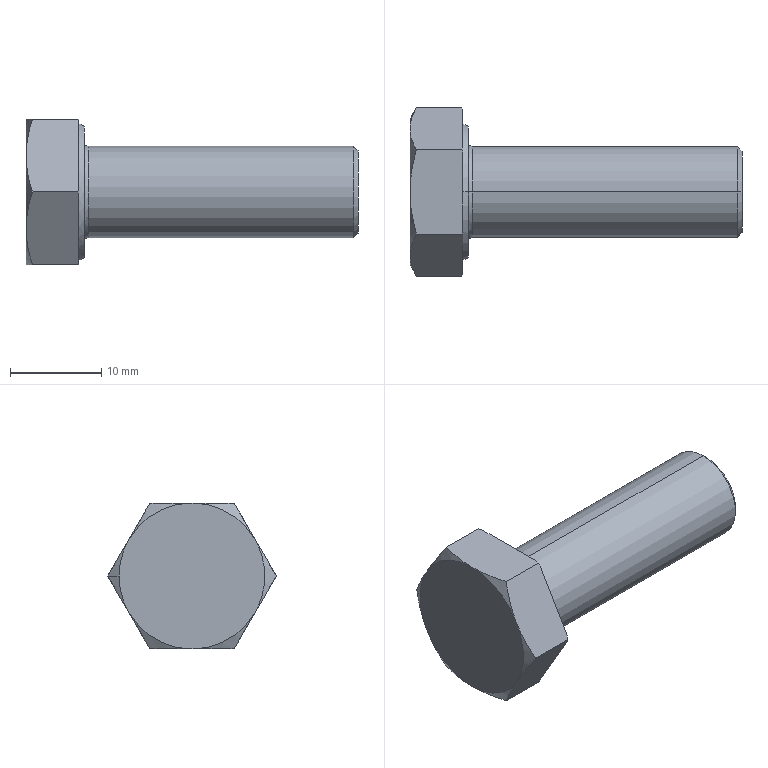Part | SolidWorks | features BaseBody 1, Chamfer 1, ICE 1 | 1 solid | 31 faces | box 36.4 x 18.475 x 16 mm | volume 3737 mm3 | cone 17 | plane 10 | spline 2 | cylinder 2 | commonest cylinder face diameters 10 x2
STEP:
#1=CARTESIAN_POINT('',(6.8,0.,-5.));
#2=VERTEX_POINT('',#1);
#3=CARTESIAN_POINT('',(6.8,0.,5.));
#4=VERTEX_POINT('',#3);
#5=CARTESIAN_POINT('',(6.8,0.,0.));
#6=DIRECTION('',(1.,0.,0.));
#7=DIRECTION('',(0.,0.,-1.));
#8=AXIS2_PLACEMENT_3D('',#5,#6,#7);
#9=CIRCLE('',#8,5.);
#10=EDGE_CURVE('',#2,#4,#9,.T.);
#11=ORIENTED_EDGE('',*,*,#10,.F.);
#12=CARTESIAN_POINT('',(6.4,0.,-5.4));
#13=VERTEX_POINT('',#12);
#14=CARTESIAN_POINT('',(6.8,0.,-5.4));
#15=DIRECTION('',(0.,-1.,0.));
#16=DIRECTION('',(0.,0.,-1.));
#17=AXIS2_PLACEMENT_3D('',#14,#15,#16);
#18=CIRCLE('',#17,0.4);
#19=EDGE_CURVE('',#2,#13,#18,.T.);
#20=ORIENTED_EDGE('',*,*,#19,.T.);
#21=CARTESIAN_POINT('',(6.4,0.,5.4));
#22=VERTEX_POINT('',#21);
#23=CARTESIAN_POINT('',(6.4,0.,5.4));
#24=CARTESIAN_POINT('',(6.4,0.1651,5.4));
#25=CARTESIAN_POINT('',(6.4,0.4117,5.389));
#26=CARTESIAN_POINT('',(6.4,0.6977,5.356));
#27=CARTESIAN_POINT('',(6.4,0.8403,5.334));
#28=CARTESIAN_POINT('',(6.4,0.9013,5.324));
#29=CARTESIAN_POINT('',(6.4,0.942,5.317));
#30=CARTESIAN_POINT('',(6.4,0.9611,5.314));
#31=CARTESIAN_POINT('',(6.4,1.155,5.278));
#32=CARTESIAN_POINT('',(6.4,1.409,5.218));
#33=CARTESIAN_POINT('',(6.4,1.7,5.127));
#34=CARTESIAN_POINT('',(6.4,1.824,5.083));
#35=CARTESIAN_POINT('',(6.4,1.906,5.053));
#36=CARTESIAN_POINT('',(6.4,1.945,5.038));
#37=CARTESIAN_POINT('',(6.4,2.157,4.954));
#38=CARTESIAN_POINT('',(6.4,2.405,4.841));
#39=CARTESIAN_POINT('',(6.4,2.644,4.709));
#40=CARTESIAN_POINT('',(6.4,2.801,4.618));
#41=CARTESIAN_POINT('',(6.4,2.877,4.571));
#42=CARTESIAN_POINT('',(6.4,3.267,4.316));
#43=CARTESIAN_POINT('',(6.4,3.555,4.082));
#44=CARTESIAN_POINT('',(6.4,3.95,3.687));
#45=CARTESIAN_POINT('',(6.4,4.137,3.48));
#46=CARTESIAN_POINT('',(6.4,4.306,3.26));
#47=CARTESIAN_POINT('',(6.4,4.416,3.11));
#48=CARTESIAN_POINT('',(6.4,4.47,3.031));
#49=CARTESIAN_POINT('',(6.4,4.62,2.802));
#50=CARTESIAN_POINT('',(6.4,4.757,2.567));
#51=CARTESIAN_POINT('',(6.4,4.896,2.281));
#52=CARTESIAN_POINT('',(6.4,4.951,2.156));
#53=CARTESIAN_POINT('',(6.4,4.987,2.072));
#54=CARTESIAN_POINT('',(6.4,5.005,2.028));
#55=CARTESIAN_POINT('',(6.4,5.085,1.825));
#56=CARTESIAN_POINT('',(6.4,5.17,1.577));
#57=CARTESIAN_POINT('',(6.4,5.247,1.282));
#58=CARTESIAN_POINT('',(6.4,5.28,1.133));
#59=CARTESIAN_POINT('',(6.4,5.293,1.069));
#60=CARTESIAN_POINT('',(6.4,5.302,1.026));
#61=CARTESIAN_POINT('',(6.4,5.306,1.003));
#62=CARTESIAN_POINT('',(6.4,5.37,0.6582));
#63=CARTESIAN_POINT('',(6.4,5.4,0.3299));
#64=CARTESIAN_POINT('',(6.4,5.4,-0.165));
#65=CARTESIAN_POINT('',(6.4,5.389,-0.4115));
#66=CARTESIAN_POINT('',(6.4,5.356,-0.6976));
#67=CARTESIAN_POINT('',(6.4,5.335,-0.8402));
#68=CARTESIAN_POINT('',(6.4,5.324,-0.9013));
#69=CARTESIAN_POINT('',(6.4,5.317,-0.9419));
#70=CARTESIAN_POINT('',(6.4,5.314,-0.9611));
#71=CARTESIAN_POINT('',(6.4,5.278,-1.155));
#72=CARTESIAN_POINT('',(6.4,5.218,-1.409));
#73=CARTESIAN_POINT('',(6.4,5.127,-1.7));
#74=CARTESIAN_POINT('',(6.4,5.083,-1.824));
#75=CARTESIAN_POINT('',(6.4,5.053,-1.906));
#76=CARTESIAN_POINT('',(6.4,5.038,-1.945));
#77=CARTESIAN_POINT('',(6.4,4.954,-2.157));
#78=CARTESIAN_POINT('',(6.4,4.841,-2.405));
#79=CARTESIAN_POINT('',(6.4,4.709,-2.644));
#80=CARTESIAN_POINT('',(6.4,4.618,-2.801));
#81=CARTESIAN_POINT('',(6.4,4.571,-2.877));
#82=CARTESIAN_POINT('',(6.4,4.316,-3.267));
#83=CARTESIAN_POINT('',(6.4,4.082,-3.555));
#84=CARTESIAN_POINT('',(6.4,3.687,-3.95));
#85=CARTESIAN_POINT('',(6.4,3.48,-4.137));
#86=CARTESIAN_POINT('',(6.4,3.26,-4.306));
#87=CARTESIAN_POINT('',(6.4,3.11,-4.416));
#88=CARTESIAN_POINT('',(6.4,3.031,-4.47));
#89=CARTESIAN_POINT('',(6.4,2.802,-4.62));
#90=CARTESIAN_POINT('',(6.4,2.567,-4.757));
#91=CARTESIAN_POINT('',(6.4,2.281,-4.896));
#92=CARTESIAN_POINT('',(6.4,2.156,-4.951));
#93=CARTESIAN_POINT('',(6.4,2.072,-4.987));
#94=CARTESIAN_POINT('',(6.4,2.028,-5.005));
#95=CARTESIAN_POINT('',(6.4,1.825,-5.085));
#96=CARTESIAN_POINT('',(6.4,1.577,-5.17));
#97=CARTESIAN_POINT('',(6.4,1.282,-5.247));
#98=CARTESIAN_POINT('',(6.4,1.133,-5.28));
#99=CARTESIAN_POINT('',(6.4,1.069,-5.293));
#100=CARTESIAN_POINT('',(6.4,1.026,-5.302));
#101=CARTESIAN_POINT('',(6.4,1.003,-5.306));
#102=CARTESIAN_POINT('',(6.4,0.658,-5.37));
#103=CARTESIAN_POINT('',(6.4,0.3305,-5.4));
#104=CARTESIAN_POINT('',(6.4,0.,-5.4));
#105=B_SPLINE_CURVE_WITH_KNOTS('',3,(#23,#24,#25,#26,#27,#28,#29,#30,#31,#32,#33,#34,#35,#36,#37,#38,#39,#40,#41,#42,#43,#44,#45,#46,#47,#48,#49,#50,#51,#52,#53,#54,#55,#56,#57,#58,#59,#60,#61,#62,#63,#64,#65,#66,#67,#68,#69,#70,#71,#72,#73,#74,#75,#76,#77,#78,#79,#80,#81,#82,#83,#84,#85,#86,#87,#88,#89,#90,#91,#92,#93,#94,#95,#96,#97,#98,#99,#100,#101,#102,#103,#104),.UNSPECIFIED.,.F.,.F.,(4,1,1,1,2,2,1,1,2,2,1,2,2,2,1,2,2,1,1,2,2,1,1,1,2,2,2,1,1,1,2,2,1,1,2,2,1,2,2,2,1,2,2,1,1,2,2,1,1,1,2,2,4),(0.,0.03125,0.04688,0.05469,0.05859,0.0625,0.09375,0.1094,0.1172,0.125,0.1563,0.1719,0.1875,0.25,0.2813,0.2969,0.3125,0.3438,0.3594,0.3672,0.375,0.4063,0.4219,0.4297,0.4336,0.4375,0.5,0.5313,0.5469,0.5547,0.5586,0.5625,0.5938,0.6094,0.6172,0.625,0.6563,0.6719,0.6875,0.75,0.7813,0.7969,0.8125,0.8438,0.8594,0.8672,0.875,0.9063,0.9219,0.9297,0.9336,0.9375,1.),.UNSPECIFIED.);
#106=EDGE_CURVE('',#22,#13,#105,.T.);
#107=ORIENTED_EDGE('',*,*,#106,.F.);
#108=CARTESIAN_POINT('',(6.8,0.,5.4));
#109=DIRECTION('',(0.,1.,0.));
#110=DIRECTION('',(0.,0.,1.));
#111=AXIS2_PLACEMENT_3D('',#108,#109,#110);
#112=CIRCLE('',#111,0.4);
#113=EDGE_CURVE('',#4,#22,#112,.T.);
#114=ORIENTED_EDGE('',*,*,#113,.F.);
#115=EDGE_LOOP('',(#11,#20,#107,#114));
#116=FACE_OUTER_BOUND('',#115,.T.);
#117=CARTESIAN_POINT('',(6.8,0.,5.));
#118=CARTESIAN_POINT('',(6.8,10.,5.));
#119=CARTESIAN_POINT('',(6.8,10.,-5.));
#120=CARTESIAN_POINT('',(6.8,0.,-5.));
#121=CARTESIAN_POINT('',(6.566,0.,5.));
#122=CARTESIAN_POINT('',(6.566,10.,5.));
#123=CARTESIAN_POINT('',(6.566,10.,-5.));
#124=CARTESIAN_POINT('',(6.566,0.,-5.));
#125=CARTESIAN_POINT('',(6.4,0.,5.166));
#126=CARTESIAN_POINT('',(6.4,10.331,5.166));
#127=CARTESIAN_POINT('',(6.4,10.331,-5.166));
#128=CARTESIAN_POINT('',(6.4,0.,-5.166));
#129=CARTESIAN_POINT('',(6.4,0.,5.4));
#130=CARTESIAN_POINT('',(6.4,10.8,5.4));
#131=CARTESIAN_POINT('',(6.4,10.8,-5.4));
#132=CARTESIAN_POINT('',(6.4,0.,-5.4));
#133=(BOUNDED_SURFACE()B_SPLINE_SURFACE(3,3,((#117,#118,#119,#120),(#121,#122,#123,#124),(#125,#126,#127,#128),(#129,#130,#131,#132)),.UNSPECIFIED.,.F.,.F.,.F.)B_SPLINE_SURFACE_WITH_KNOTS((4,4),(4,4),(0.,1.),(0.,1.),.UNSPECIFIED.)GEOMETRIC_REPRESENTATION_ITEM()RATIONAL_B_SPLINE_SURFACE(((1.,0.3333,0.3333,1.),(0.8047,0.2682,0.2682,0.8047),(0.8047,0.2682,0.2682,0.8047),(1.,0.3333,0.3333,1.)))REPRESENTATION_ITEM('')SURFACE());
#134=ADVANCED_FACE('',(#116),#133,.F.);
#135=CARTESIAN_POINT('',(36.4,0.,-4.5));
#136=VERTEX_POINT('',#135);
#137=CARTESIAN_POINT('',(36.4,0.,4.5));
#138=VERTEX_POINT('',#137);
#139=CARTESIAN_POINT('',(36.4,0.,0.));
#140=DIRECTION('',(1.,0.,0.));
#141=DIRECTION('',(0.,0.,-1.));
#142=AXIS2_PLACEMENT_3D('',#139,#140,#141);
#143=CIRCLE('',#142,4.5);
#144=EDGE_CURVE('',#136,#138,#143,.T.);
#145=ORIENTED_EDGE('',*,*,#144,.F.);
#146=CARTESIAN_POINT('',(35.9,0.,-5.));
#147=VERTEX_POINT('',#146);
#148=CARTESIAN_POINT('',(35.9,0.,-5.));
#149=DIRECTION('',(-0.7071,0.,-0.7071));
#150=VECTOR('',#149,1000.);
#151=LINE('',#148,#150);
#152=EDGE_CURVE('',#136,#147,#151,.T.);
#153=ORIENTED_EDGE('',*,*,#152,.T.);
#154=CARTESIAN_POINT('',(35.9,0.,5.));
#155=VERTEX_POINT('',#154);
#156=CARTESIAN_POINT('',(35.9,0.,0.));
#157=DIRECTION('',(-1.,0.,0.));
#158=DIRECTION('',(0.,0.,-1.));
#159=AXIS2_PLACEMENT_3D('',#156,#157,#158);
#160=CIRCLE('',#159,5.);
#161=EDGE_CURVE('',#155,#147,#160,.T.);
#162=ORIENTED_EDGE('',*,*,#161,.F.);
#163=CARTESIAN_POINT('',(35.9,0.,5.));
#164=DIRECTION('',(-0.7071,0.,0.7071));
#165=VECTOR('',#164,1000.);
#166=LINE('',#163,#165);
#167=EDGE_CURVE('',#138,#155,#166,.T.);
#168=ORIENTED_EDGE('',*,*,#167,.F.);
#169=EDGE_LOOP('',(#145,#153,#162,#168));
#170=FACE_OUTER_BOUND('',#169,.T.);
#171=CARTESIAN_POINT('',(35.9,0.,0.));
#172=DIRECTION('',(-1.,0.,0.));
#173=DIRECTION('',(0.,0.,1.));
#174=AXIS2_PLACEMENT_3D('',#171,#172,#173);
#175=CONICAL_SURFACE('',#174,5.,0.7854);
#176=ADVANCED_FACE('',(#170),#175,.T.);
#177=CARTESIAN_POINT('',(6.4,0.,-7.177));
#178=VERTEX_POINT('',#177);
#179=CARTESIAN_POINT('',(6.4,0.,7.177));
#180=VERTEX_POINT('',#179);
#181=CARTESIAN_POINT('',(6.4,0.,0.));
#182=DIRECTION('',(1.,0.,0.));
#183=DIRECTION('',(0.,0.,1.));
#184=AXIS2_PLACEMENT_3D('',#181,#182,#183);
#185=CIRCLE('',#184,7.177);
#186=EDGE_CURVE('',#178,#180,#185,.T.);
#187=ORIENTED_EDGE('',*,*,#186,.F.);
#188=CARTESIAN_POINT('',(5.8,0.,-7.524));
#189=VERTEX_POINT('',#188);
#190=CARTESIAN_POINT('',(5.8,0.,-7.524));
#191=DIRECTION('',(-0.866,0.,-0.5));
#192=VECTOR('',#191,1000.);
#193=LINE('',#190,#192);
#194=EDGE_CURVE('',#178,#189,#193,.T.);
#195=ORIENTED_EDGE('',*,*,#194,.T.);
#196=CARTESIAN_POINT('',(5.8,0.,7.524));
#197=VERTEX_POINT('',#196);
#198=CARTESIAN_POINT('',(5.8,0.,0.));
#199=DIRECTION('',(1.,0.,0.));
#200=DIRECTION('',(0.,0.,1.));
#201=AXIS2_PLACEMENT_3D('',#198,#199,#200);
#202=CIRCLE('',#201,7.524);
#203=EDGE_CURVE('',#189,#197,#202,.T.);
#204=ORIENTED_EDGE('',*,*,#203,.T.);
#205=CARTESIAN_POINT('',(5.8,0.,7.524));
#206=DIRECTION('',(-0.866,0.,0.5));
#207=VECTOR('',#206,1000.);
#208=LINE('',#205,#207);
#209=EDGE_CURVE('',#180,#197,#208,.T.);
#210=ORIENTED_EDGE('',*,*,#209,.F.);
#211=EDGE_LOOP('',(#187,#195,#204,#210));
#212=FACE_OUTER_BOUND('',#211,.T.);
#213=CARTESIAN_POINT('',(5.8,0.,0.));
#214=DIRECTION('',(-1.,0.,0.));
#215=DIRECTION('',(0.,0.,1.));
#216=AXIS2_PLACEMENT_3D('',#213,#214,#215);
#217=CONICAL_SURFACE('',#216,7.524,0.5236);
#218=ADVANCED_FACE('',(#212),#217,.T.);
#219=CARTESIAN_POINT('',(0.,6.928,-4.));
#220=VERTEX_POINT('',#219);
#221=CARTESIAN_POINT('',(0.,8.,0.));
#222=VERTEX_POINT('',#221);
#223=CARTESIAN_POINT('',(0.,0.,0.));
#224=DIRECTION('',(1.,0.,0.));
#225=DIRECTION('',(0.,1.,0.));
#226=AXIS2_PLACEMENT_3D('',#223,#224,#225);
#227=CIRCLE('',#226,8.);
#228=EDGE_CURVE('',#220,#222,#227,.T.);
#229=ORIENTED_EDGE('',*,*,#228,.T.);
#230=CARTESIAN_POINT('',(0.7145,9.238,0.));
#231=VERTEX_POINT('',#230);
#232=CARTESIAN_POINT('',(0.7188,9.245,0.));
#233=DIRECTION('',(0.5,0.866,0.));
#234=VECTOR('',#233,1000.);
#235=LINE('',#232,#234);
#236=EDGE_CURVE('',#222,#231,#235,.T.);
#237=ORIENTED_EDGE('',*,*,#236,.T.);
#238=CARTESIAN_POINT('',(0.7145,9.238,0.));
#239=CARTESIAN_POINT('',(0.4967,8.86,-0.6534));
#240=CARTESIAN_POINT('',(0.3171,8.48,-1.312));
#241=CARTESIAN_POINT('',(0.06831,7.711,-2.644));
#242=CARTESIAN_POINT('',(0.,7.322,-3.317));
#243=CARTESIAN_POINT('',(0.,6.928,-4.));
#244=B_SPLINE_CURVE_WITH_KNOTS('',3,(#238,#239,#240,#241,#242,#243),.UNSPECIFIED.,.F.,.F.,(4,2,4),(0.,0.002337,0.004674),.UNSPECIFIED.);
#245=EDGE_CURVE('',#231,#220,#244,.T.);
#246=ORIENTED_EDGE('',*,*,#245,.T.);
#247=EDGE_LOOP('',(#229,#237,#246));
#248=FACE_OUTER_BOUND('',#247,.T.);
#249=CARTESIAN_POINT('',(0.7188,0.,0.));
#250=DIRECTION('',(1.,0.,0.));
#251=DIRECTION('',(0.,1.,0.));
#252=AXIS2_PLACEMENT_3D('',#249,#250,#251);
#253=CONICAL_SURFACE('',#252,9.245,1.047);
#254=ADVANCED_FACE('',(#248),#253,.T.);
#255=ORIENTED_EDGE('',*,*,#10,.T.);
#256=CARTESIAN_POINT('',(0.,0.,5.));
#257=DIRECTION('',(1.,0.,0.));
#258=VECTOR('',#257,1000.);
#259=LINE('',#256,#258);
#260=EDGE_CURVE('',#4,#155,#259,.T.);
#261=ORIENTED_EDGE('',*,*,#260,.T.);
#262=ORIENTED_EDGE('',*,*,#161,.T.);
#263=CARTESIAN_POINT('',(0.,0.,-5.));
#264=DIRECTION('',(1.,0.,0.));
#265=VECTOR('',#264,1000.);
#266=LINE('',#263,#265);
#267=EDGE_CURVE('',#2,#147,#266,.T.);
#268=ORIENTED_EDGE('',*,*,#267,.F.);
#269=EDGE_LOOP('',(#255,#261,#262,#268));
#270=FACE_OUTER_BOUND('',#269,.T.);
#271=CARTESIAN_POINT('',(0.,0.,0.));
#272=DIRECTION('',(1.,0.,0.));
#273=DIRECTION('',(0.,0.,-1.));
#274=AXIS2_PLACEMENT_3D('',#271,#272,#273);
#275=CYLINDRICAL_SURFACE('',#274,5.);
#276=ADVANCED_FACE('',(#270),#275,.T.);
#277=ORIENTED_EDGE('',*,*,#260,.F.);
#278=CARTESIAN_POINT('',(6.8,0.,0.));
#279=DIRECTION('',(1.,0.,0.));
#280=DIRECTION('',(0.,0.,-1.));
#281=AXIS2_PLACEMENT_3D('',#278,#279,#280);
#282=CIRCLE('',#281,5.);
#283=EDGE_CURVE('',#4,#2,#282,.T.);
#284=ORIENTED_EDGE('',*,*,#283,.T.);
#285=ORIENTED_EDGE('',*,*,#267,.T.);
#286=CARTESIAN_POINT('',(35.9,0.,0.));
#287=DIRECTION('',(-1.,0.,0.));
#288=DIRECTION('',(0.,0.,-1.));
#289=AXIS2_PLACEMENT_3D('',#286,#287,#288);
#290=CIRCLE('',#289,5.);
#291=EDGE_CURVE('',#147,#155,#290,.T.);
#292=ORIENTED_EDGE('',*,*,#291,.T.);
#293=EDGE_LOOP('',(#277,#284,#285,#292));
#294=FACE_OUTER_BOUND('',#293,.T.);
#295=CARTESIAN_POINT('',(0.,0.,0.));
#296=DIRECTION('',(1.,0.,0.));
#297=DIRECTION('',(0.,0.,-1.));
#298=AXIS2_PLACEMENT_3D('',#295,#296,#297);
#299=CYLINDRICAL_SURFACE('',#298,5.);
#300=ADVANCED_FACE('',(#294),#299,.T.);
#301=ORIENTED_EDGE('',*,*,#19,.F.);
#302=ORIENTED_EDGE('',*,*,#283,.F.);
#303=ORIENTED_EDGE('',*,*,#113,.T.);
#304=CARTESIAN_POINT('',(6.4,0.,-5.4));
#305=CARTESIAN_POINT('',(6.4,-0.1651,-5.4));
#306=CARTESIAN_POINT('',(6.4,-0.4117,-5.389));
#307=CARTESIAN_POINT('',(6.4,-0.6977,-5.356));
#308=CARTESIAN_POINT('',(6.4,-0.8403,-5.334));
#309=CARTESIAN_POINT('',(6.4,-0.9013,-5.324));
#310=CARTESIAN_POINT('',(6.4,-0.942,-5.317));
#311=CARTESIAN_POINT('',(6.4,-0.9611,-5.314));
#312=CARTESIAN_POINT('',(6.4,-1.155,-5.278));
#313=CARTESIAN_POINT('',(6.4,-1.409,-5.218));
#314=CARTESIAN_POINT('',(6.4,-1.7,-5.127));
#315=CARTESIAN_POINT('',(6.4,-1.824,-5.083));
#316=CARTESIAN_POINT('',(6.4,-1.906,-5.053));
#317=CARTESIAN_POINT('',(6.4,-1.945,-5.038));
#318=CARTESIAN_POINT('',(6.4,-2.157,-4.954));
#319=CARTESIAN_POINT('',(6.4,-2.405,-4.841));
#320=CARTESIAN_POINT('',(6.4,-2.644,-4.709));
#321=CARTESIAN_POINT('',(6.4,-2.801,-4.618));
#322=CARTESIAN_POINT('',(6.4,-2.877,-4.571));
#323=CARTESIAN_POINT('',(6.4,-3.267,-4.316));
#324=CARTESIAN_POINT('',(6.4,-3.555,-4.082));
#325=CARTESIAN_POINT('',(6.4,-3.95,-3.687));
#326=CARTESIAN_POINT('',(6.4,-4.137,-3.48));
#327=CARTESIAN_POINT('',(6.4,-4.306,-3.26));
#328=CARTESIAN_POINT('',(6.4,-4.416,-3.11));
#329=CARTESIAN_POINT('',(6.4,-4.47,-3.031));
#330=CARTESIAN_POINT('',(6.4,-4.62,-2.802));
#331=CARTESIAN_POINT('',(6.4,-4.757,-2.567));
#332=CARTESIAN_POINT('',(6.4,-4.896,-2.281));
#333=CARTESIAN_POINT('',(6.4,-4.951,-2.156));
#334=CARTESIAN_POINT('',(6.4,-4.987,-2.072));
#335=CARTESIAN_POINT('',(6.4,-5.005,-2.028));
#336=CARTESIAN_POINT('',(6.4,-5.085,-1.825));
#337=CARTESIAN_POINT('',(6.4,-5.17,-1.577));
#338=CARTESIAN_POINT('',(6.4,-5.247,-1.282));
#339=CARTESIAN_POINT('',(6.4,-5.28,-1.133));
#340=CARTESIAN_POINT('',(6.4,-5.293,-1.069));
#341=CARTESIAN_POINT('',(6.4,-5.302,-1.026));
#342=CARTESIAN_POINT('',(6.4,-5.306,-1.003));
#343=CARTESIAN_POINT('',(6.4,-5.37,-0.6582));
#344=CARTESIAN_POINT('',(6.4,-5.4,-0.3299));
#345=CARTESIAN_POINT('',(6.4,-5.4,0.165));
#346=CARTESIAN_POINT('',(6.4,-5.389,0.4115));
#347=CARTESIAN_POINT('',(6.4,-5.356,0.6976));
#348=CARTESIAN_POINT('',(6.4,-5.335,0.8402));
#349=CARTESIAN_POINT('',(6.4,-5.324,0.9013));
#350=CARTESIAN_POINT('',(6.4,-5.317,0.9419));
#351=CARTESIAN_POINT('',(6.4,-5.314,0.9611));
#352=CARTESIAN_POINT('',(6.4,-5.278,1.155));
#353=CARTESIAN_POINT('',(6.4,-5.218,1.409));
#354=CARTESIAN_POINT('',(6.4,-5.127,1.7));
#355=CARTESIAN_POINT('',(6.4,-5.083,1.824));
#356=CARTESIAN_POINT('',(6.4,-5.053,1.906));
#357=CARTESIAN_POINT('',(6.4,-5.038,1.945));
#358=CARTESIAN_POINT('',(6.4,-4.954,2.157));
#359=CARTESIAN_POINT('',(6.4,-4.841,2.405));
#360=CARTESIAN_POINT('',(6.4,-4.709,2.644));
#361=CARTESIAN_POINT('',(6.4,-4.618,2.801));
#362=CARTESIAN_POINT('',(6.4,-4.571,2.877));
#363=CARTESIAN_POINT('',(6.4,-4.316,3.267));
#364=CARTESIAN_POINT('',(6.4,-4.082,3.555));
#365=CARTESIAN_POINT('',(6.4,-3.687,3.95));
#366=CARTESIAN_POINT('',(6.4,-3.48,4.137));
#367=CARTESIAN_POINT('',(6.4,-3.26,4.306));
#368=CARTESIAN_POINT('',(6.4,-3.11,4.416));
#369=CARTESIAN_POINT('',(6.4,-3.031,4.47));
#370=CARTESIAN_POINT('',(6.4,-2.802,4.62));
#371=CARTESIAN_POINT('',(6.4,-2.567,4.757));
#372=CARTESIAN_POINT('',(6.4,-2.281,4.896));
#373=CARTESIAN_POINT('',(6.4,-2.156,4.951));
#374=CARTESIAN_POINT('',(6.4,-2.072,4.987));
#375=CARTESIAN_POINT('',(6.4,-2.028,5.005));
#376=CARTESIAN_POINT('',(6.4,-1.825,5.085));
#377=CARTESIAN_POINT('',(6.4,-1.577,5.17));
#378=CARTESIAN_POINT('',(6.4,-1.282,5.247));
#379=CARTESIAN_POINT('',(6.4,-1.133,5.28));
#380=CARTESIAN_POINT('',(6.4,-1.069,5.293));
#381=CARTESIAN_POINT('',(6.4,-1.026,5.302));
#382=CARTESIAN_POINT('',(6.4,-1.003,5.306));
#383=CARTESIAN_POINT('',(6.4,-0.658,5.37));
#384=CARTESIAN_POINT('',(6.4,-0.3305,5.4));
#385=CARTESIAN_POINT('',(6.4,0.,5.4));
#386=B_SPLINE_CURVE_WITH_KNOTS('',3,(#304,#305,#306,#307,#308,#309,#310,#311,#312,#313,#314,#315,#316,#317,#318,#319,#320,#321,#322,#323,#324,#325,#326,#327,#328,#329,#330,#331,#332,#333,#334,#335,#336,#337,#338,#339,#340,#341,#342,#343,#344,#345,#346,#347,#348,#349,#350,#351,#352,#353,#354,#355,#356,#357,#358,#359,#360,#361,#362,#363,#364,#365,#366,#367,#368,#369,#370,#371,#372,#373,#374,#375,#376,#377,#378,#379,#380,#381,#382,#383,#384,#385),.UNSPECIFIED.,.F.,.F.,(4,1,1,1,2,2,1,1,2,2,1,2,2,2,1,2,2,1,1,2,2,1,1,1,2,2,2,1,1,1,2,2,1,1,2,2,1,2,2,2,1,2,2,1,1,2,2,1,1,1,2,2,4),(0.,0.03125,0.04688,0.05469,0.05859,0.0625,0.09375,0.1094,0.1172,0.125,0.1563,0.1719,0.1875,0.25,0.2813,0.2969,0.3125,0.3438,0.3594,0.3672,0.375,0.4063,0.4219,0.4297,0.4336,0.4375,0.5,0.5313,0.5469,0.5547,0.5586,0.5625,0.5938,0.6094,0.6172,0.625,0.6563,0.6719,0.6875,0.75,0.7812,0.7969,0.8125,0.8437,0.8594,0.8672,0.875,0.9062,0.9219,0.9297,0.9336,0.9375,1.),.UNSPECIFIED.);
#387=EDGE_CURVE('',#13,#22,#386,.T.);
#388=ORIENTED_EDGE('',*,*,#387,.F.);
#389=EDGE_LOOP('',(#301,#302,#303,#388));
#390=FACE_OUTER_BOUND('',#389,.T.);
#391=CARTESIAN_POINT('',(6.8,0.,-5.));
#392=CARTESIAN_POINT('',(6.8,-10.,-5.));
#393=CARTESIAN_POINT('',(6.8,-10.,5.));
#394=CARTESIAN_POINT('',(6.8,0.,5.));
#395=CARTESIAN_POINT('',(6.566,0.,-5.));
#396=CARTESIAN_POINT('',(6.566,-10.,-5.));
#397=CARTESIAN_POINT('',(6.566,-10.,5.));
#398=CARTESIAN_POINT('',(6.566,0.,5.));
#399=CARTESIAN_POINT('',(6.4,0.,-5.166));
#400=CARTESIAN_POINT('',(6.4,-10.331,-5.166));
#401=CARTESIAN_POINT('',(6.4,-10.331,5.166));
#402=CARTESIAN_POINT('',(6.4,0.,5.166));
#403=CARTESIAN_POINT('',(6.4,0.,-5.4));
#404=CARTESIAN_POINT('',(6.4,-10.8,-5.4));
#405=CARTESIAN_POINT('',(6.4,-10.8,5.4));
#406=CARTESIAN_POINT('',(6.4,0.,5.4));
#407=(BOUNDED_SURFACE()B_SPLINE_SURFACE(3,3,((#391,#392,#393,#394),(#395,#396,#397,#398),(#399,#400,#401,#402),(#403,#404,#405,#406)),.UNSPECIFIED.,.F.,.F.,.F.)B_SPLINE_SURFACE_WITH_KNOTS((4,4),(4,4),(0.,1.),(0.,1.),.UNSPECIFIED.)GEOMETRIC_REPRESENTATION_ITEM()RATIONAL_B_SPLINE_SURFACE(((1.,0.3333,0.3333,1.),(0.8047,0.2682,0.2682,0.8047),(0.8047,0.2682,0.2682,0.8047),(1.,0.3333,0.3333,1.)))REPRESENTATION_ITEM('')SURFACE());
#408=ADVANCED_FACE('',(#390),#407,.F.);
#409=ORIENTED_EDGE('',*,*,#106,.T.);
#410=ORIENTED_EDGE('',*,*,#387,.T.);
#411=EDGE_LOOP('',(#409,#410));
#412=FACE_BOUND('',#411,.T.);
#413=CARTESIAN_POINT('',(6.4,0.,0.));
#414=DIRECTION('',(1.,0.,0.));
#415=DIRECTION('',(0.,0.,1.));
#416=AXIS2_PLACEMENT_3D('',#413,#414,#415);
#417=CIRCLE('',#416,7.177);
#418=EDGE_CURVE('',#180,#178,#417,.T.);
#419=ORIENTED_EDGE('',*,*,#418,.T.);
#420=ORIENTED_EDGE('',*,*,#186,.T.);
#421=EDGE_LOOP('',(#419,#420));
#422=FACE_OUTER_BOUND('',#421,.T.);
#423=CARTESIAN_POINT('',(6.4,9.238,0.));
#424=DIRECTION('',(1.,0.,0.));
#425=DIRECTION('',(0.,0.,-1.));
#426=AXIS2_PLACEMENT_3D('',#423,#424,#425);
#427=PLANE('',#426);
#428=ADVANCED_FACE('',(#412,#422),#427,.T.);
#429=ORIENTED_EDGE('',*,*,#194,.F.);
#430=ORIENTED_EDGE('',*,*,#418,.F.);
#431=ORIENTED_EDGE('',*,*,#209,.T.);
#432=CARTESIAN_POINT('',(5.8,0.,0.));
#433=DIRECTION('',(1.,0.,0.));
#434=DIRECTION('',(0.,0.,1.));
#435=AXIS2_PLACEMENT_3D('',#432,#433,#434);
#436=CIRCLE('',#435,7.524);
#437=EDGE_CURVE('',#197,#189,#436,.T.);
#438=ORIENTED_EDGE('',*,*,#437,.T.);
#439=EDGE_LOOP('',(#429,#430,#431,#438));
#440=FACE_OUTER_BOUND('',#439,.T.);
#441=CARTESIAN_POINT('',(5.8,0.,0.));
#442=DIRECTION('',(-1.,0.,0.));
#443=DIRECTION('',(0.,0.,1.));
#444=AXIS2_PLACEMENT_3D('',#441,#442,#443);
#445=CONICAL_SURFACE('',#444,7.524,0.5236);
#446=ADVANCED_FACE('',(#440),#445,.T.);
#447=ORIENTED_EDGE('',*,*,#437,.F.);
#448=ORIENTED_EDGE('',*,*,#203,.F.);
#449=EDGE_LOOP('',(#447,#448));
#450=FACE_BOUND('',#449,.T.);
#451=CARTESIAN_POINT('',(5.8,4.208,8.));
#452=VERTEX_POINT('',#451);
#453=CARTESIAN_POINT('',(5.8,-4.208,8.));
#454=VERTEX_POINT('',#453);
#455=CARTESIAN_POINT('',(5.8,7.524,8.));
#456=DIRECTION('',(0.,-1.,0.));
#457=VECTOR('',#456,1000.);
#458=LINE('',#455,#457);
#459=EDGE_CURVE('',#452,#454,#458,.T.);
#460=ORIENTED_EDGE('',*,*,#459,.T.);
#461=CARTESIAN_POINT('',(5.8,-4.824,7.644));
#462=VERTEX_POINT('',#461);
#463=CARTESIAN_POINT('',(5.8,0.,0.));
#464=DIRECTION('',(1.,0.,0.));
#465=DIRECTION('',(0.,0.,1.));
#466=AXIS2_PLACEMENT_3D('',#463,#464,#465);
#467=CIRCLE('',#466,9.039);
#468=EDGE_CURVE('',#454,#462,#467,.T.);
#469=ORIENTED_EDGE('',*,*,#468,.T.);
#470=CARTESIAN_POINT('',(5.8,-9.032,0.3557));
#471=VERTEX_POINT('',#470);
#472=CARTESIAN_POINT('',(5.8,-4.824,7.644));
#473=DIRECTION('',(0.,-0.5,-0.866));
#474=VECTOR('',#473,1000.);
#475=LINE('',#472,#474);
#476=EDGE_CURVE('',#462,#471,#475,.T.);
#477=ORIENTED_EDGE('',*,*,#476,.T.);
#478=CARTESIAN_POINT('',(5.8,-9.032,-0.3557));
#479=VERTEX_POINT('',#478);
#480=CARTESIAN_POINT('',(5.8,0.,0.));
#481=DIRECTION('',(1.,0.,0.));
#482=DIRECTION('',(0.,0.,1.));
#483=AXIS2_PLACEMENT_3D('',#480,#481,#482);
#484=CIRCLE('',#483,9.039);
#485=EDGE_CURVE('',#471,#479,#484,.T.);
#486=ORIENTED_EDGE('',*,*,#485,.T.);
#487=CARTESIAN_POINT('',(5.8,-4.824,-7.644));
#488=VERTEX_POINT('',#487);
#489=CARTESIAN_POINT('',(5.8,-9.032,-0.3557));
#490=DIRECTION('',(0.,0.5,-0.866));
#491=VECTOR('',#490,1000.);
#492=LINE('',#489,#491);
#493=EDGE_CURVE('',#479,#488,#492,.T.);
#494=ORIENTED_EDGE('',*,*,#493,.T.);
#495=CARTESIAN_POINT('',(5.8,-4.208,-8.));
#496=VERTEX_POINT('',#495);
#497=CARTESIAN_POINT('',(5.8,0.,0.));
#498=DIRECTION('',(1.,0.,0.));
#499=DIRECTION('',(0.,0.,1.));
#500=AXIS2_PLACEMENT_3D('',#497,#498,#499);
#501=CIRCLE('',#500,9.039);
#502=EDGE_CURVE('',#488,#496,#501,.T.);
#503=ORIENTED_EDGE('',*,*,#502,.T.);
#504=CARTESIAN_POINT('',(5.8,4.208,-8.));
#505=VERTEX_POINT('',#504);
#506=CARTESIAN_POINT('',(5.8,7.524,-8.));
#507=DIRECTION('',(0.,1.,0.));
#508=VECTOR('',#507,1000.);
#509=LINE('',#506,#508);
#510=EDGE_CURVE('',#496,#505,#509,.T.);
#511=ORIENTED_EDGE('',*,*,#510,.T.);
#512=CARTESIAN_POINT('',(5.8,4.824,-7.644));
#513=VERTEX_POINT('',#512);
#514=CARTESIAN_POINT('',(5.8,0.,0.));
#515=DIRECTION('',(1.,0.,0.));
#516=DIRECTION('',(0.,0.,1.));
#517=AXIS2_PLACEMENT_3D('',#514,#515,#516);
#518=CIRCLE('',#517,9.039);
#519=EDGE_CURVE('',#505,#513,#518,.T.);
#520=ORIENTED_EDGE('',*,*,#519,.T.);
#521=CARTESIAN_POINT('',(5.8,9.032,-0.3557));
#522=VERTEX_POINT('',#521);
#523=CARTESIAN_POINT('',(5.8,4.824,-7.644));
#524=DIRECTION('',(0.,0.5,0.866));
#525=VECTOR('',#524,1000.);
#526=LINE('',#523,#525);
#527=EDGE_CURVE('',#513,#522,#526,.T.);
#528=ORIENTED_EDGE('',*,*,#527,.T.);
#529=CARTESIAN_POINT('',(5.8,9.032,0.3557));
#530=VERTEX_POINT('',#529);
#531=CARTESIAN_POINT('',(5.8,0.,0.));
#532=DIRECTION('',(1.,0.,0.));
#533=DIRECTION('',(0.,0.,1.));
#534=AXIS2_PLACEMENT_3D('',#531,#532,#533);
#535=CIRCLE('',#534,9.039);
#536=EDGE_CURVE('',#522,#530,#535,.T.);
#537=ORIENTED_EDGE('',*,*,#536,.T.);
#538=CARTESIAN_POINT('',(5.8,4.824,7.644));
#539=VERTEX_POINT('',#538);
#540=CARTESIAN_POINT('',(5.8,9.032,0.3557));
#541=DIRECTION('',(0.,-0.5,0.866));
#542=VECTOR('',#541,1000.);
#543=LINE('',#540,#542);
#544=EDGE_CURVE('',#530,#539,#543,.T.);
#545=ORIENTED_EDGE('',*,*,#544,.T.);
#546=CARTESIAN_POINT('',(5.8,0.,0.));
#547=DIRECTION('',(1.,0.,0.));
#548=DIRECTION('',(0.,0.,1.));
#549=AXIS2_PLACEMENT_3D('',#546,#547,#548);
#550=CIRCLE('',#549,9.039);
#551=EDGE_CURVE('',#539,#452,#550,.T.);
#552=ORIENTED_EDGE('',*,*,#551,.T.);
#553=EDGE_LOOP('',(#460,#469,#477,#486,#494,#503,#511,#520,#528,#537,#545,#552));
#554=FACE_OUTER_BOUND('',#553,.T.);
#555=CARTESIAN_POINT('',(5.8,7.524,0.));
#556=DIRECTION('',(1.,0.,0.));
#557=DIRECTION('',(0.,0.,-1.));
#558=AXIS2_PLACEMENT_3D('',#555,#556,#557);
#559=PLANE('',#558);
#560=ADVANCED_FACE('',(#450,#554),#559,.T.);
#561=ORIENTED_EDGE('',*,*,#468,.F.);
#562=CARTESIAN_POINT('',(5.685,-4.619,8.));
#563=VERTEX_POINT('',#562);
#564=CARTESIAN_POINT('',(5.8,-4.208,8.));
#565=CARTESIAN_POINT('',(5.763,-4.344,8.));
#566=CARTESIAN_POINT('',(5.725,-4.481,8.));
#567=CARTESIAN_POINT('',(5.685,-4.619,8.));
#568=B_SPLINE_CURVE_WITH_KNOTS('',3,(#564,#565,#566,#567),.UNSPECIFIED.,.F.,.F.,(4,4),(0.,1.),.UNSPECIFIED.);
#569=EDGE_CURVE('',#454,#563,#568,.T.);
#570=ORIENTED_EDGE('',*,*,#569,.T.);
#571=CARTESIAN_POINT('',(5.685,-4.619,8.));
#572=CARTESIAN_POINT('',(5.725,-4.688,7.881));
#573=CARTESIAN_POINT('',(5.763,-4.756,7.762));
#574=CARTESIAN_POINT('',(5.8,-4.824,7.644));
#575=B_SPLINE_CURVE_WITH_KNOTS('',3,(#571,#572,#573,#574),.UNSPECIFIED.,.F.,.F.,(4,4),(0.000000524,1.),.UNSPECIFIED.);
#576=EDGE_CURVE('',#563,#462,#575,.T.);
#577=ORIENTED_EDGE('',*,*,#576,.T.);
#578=EDGE_LOOP('',(#561,#570,#577));
#579=FACE_OUTER_BOUND('',#578,.T.);
#580=CARTESIAN_POINT('',(5.685,0.,0.));
#581=DIRECTION('',(-1.,0.,0.));
#582=DIRECTION('',(0.,0.,1.));
#583=AXIS2_PLACEMENT_3D('',#580,#581,#582);
#584=CONICAL_SURFACE('',#583,9.239,1.047);
#585=ADVANCED_FACE('',(#579),#584,.T.);
#586=CARTESIAN_POINT('',(5.685,4.619,8.));
#587=VERTEX_POINT('',#586);
#588=CARTESIAN_POINT('',(5.685,4.619,8.));
#589=CARTESIAN_POINT('',(5.725,4.481,8.));
#590=CARTESIAN_POINT('',(5.763,4.344,8.));
#591=CARTESIAN_POINT('',(5.8,4.208,8.));
#592=B_SPLINE_CURVE_WITH_KNOTS('',3,(#588,#589,#590,#591),.UNSPECIFIED.,.F.,.F.,(4,4),(0.,1.),.UNSPECIFIED.);
#593=EDGE_CURVE('',#587,#452,#592,.T.);
#594=ORIENTED_EDGE('',*,*,#593,.F.);
#595=CARTESIAN_POINT('',(0.7145,4.619,8.));
#596=VERTEX_POINT('',#595);
#597=CARTESIAN_POINT('',(6.4,4.619,8.));
#598=DIRECTION('',(1.,0.,0.));
#599=VECTOR('',#598,1000.);
#600=LINE('',#597,#599);
#601=EDGE_CURVE('',#596,#587,#600,.T.);
#602=ORIENTED_EDGE('',*,*,#601,.F.);
#603=CARTESIAN_POINT('',(0.,0.,8.));
#604=VERTEX_POINT('',#603);
#605=CARTESIAN_POINT('',(0.,0.,8.));
#606=CARTESIAN_POINT('',(0.,0.7882,8.));
#607=CARTESIAN_POINT('',(0.06831,1.566,8.));
#608=CARTESIAN_POINT('',(0.3171,3.104,8.));
#609=CARTESIAN_POINT('',(0.4967,3.864,8.));
#610=CARTESIAN_POINT('',(0.7145,4.619,8.));
#611=B_SPLINE_CURVE_WITH_KNOTS('',3,(#605,#606,#607,#608,#609,#610),.UNSPECIFIED.,.F.,.F.,(4,2,4),(0.,0.002337,0.004674),.UNSPECIFIED.);
#612=EDGE_CURVE('',#604,#596,#611,.T.);
#613=ORIENTED_EDGE('',*,*,#612,.F.);
#614=CARTESIAN_POINT('',(0.7145,-4.619,8.));
#615=VERTEX_POINT('',#614);
#616=CARTESIAN_POINT('',(0.7145,-4.619,8.));
#617=CARTESIAN_POINT('',(0.4967,-3.864,8.));
#618=CARTESIAN_POINT('',(0.3171,-3.104,8.));
#619=CARTESIAN_POINT('',(0.06831,-1.566,8.));
#620=CARTESIAN_POINT('',(0.,-0.7882,8.));
#621=CARTESIAN_POINT('',(0.,0.,8.));
#622=B_SPLINE_CURVE_WITH_KNOTS('',3,(#616,#617,#618,#619,#620,#621),.UNSPECIFIED.,.F.,.F.,(4,2,4),(0.,0.002337,0.004674),.UNSPECIFIED.);
#623=EDGE_CURVE('',#615,#604,#622,.T.);
#624=ORIENTED_EDGE('',*,*,#623,.F.);
#625=CARTESIAN_POINT('',(6.4,-4.619,8.));
#626=DIRECTION('',(-1.,0.,0.));
#627=VECTOR('',#626,1000.);
#628=LINE('',#625,#627);
#629=EDGE_CURVE('',#563,#615,#628,.T.);
#630=ORIENTED_EDGE('',*,*,#629,.F.);
#631=ORIENTED_EDGE('',*,*,#569,.F.);
#632=ORIENTED_EDGE('',*,*,#459,.F.);
#633=EDGE_LOOP('',(#594,#602,#613,#624,#630,#631,#632));
#634=FACE_OUTER_BOUND('',#633,.T.);
#635=CARTESIAN_POINT('',(6.4,4.619,8.));
#636=DIRECTION('',(0.,0.,-1.));
#637=DIRECTION('',(-1.,0.,0.));
#638=AXIS2_PLACEMENT_3D('',#635,#636,#637);
#639=PLANE('',#638);
#640=ADVANCED_FACE('',(#634),#639,.F.);
#641=ORIENTED_EDGE('',*,*,#551,.F.);
#642=CARTESIAN_POINT('',(5.8,4.824,7.644));
#643=CARTESIAN_POINT('',(5.763,4.756,7.762));
#644=CARTESIAN_POINT('',(5.725,4.688,7.881));
#645=CARTESIAN_POINT('',(5.685,4.619,8.));
#646=B_SPLINE_CURVE_WITH_KNOTS('',3,(#642,#643,#644,#645),.UNSPECIFIED.,.F.,.F.,(4,4),(0.,1.),.UNSPECIFIED.);
#647=EDGE_CURVE('',#539,#587,#646,.T.);
#648=ORIENTED_EDGE('',*,*,#647,.T.);
#649=ORIENTED_EDGE('',*,*,#593,.T.);
#650=EDGE_LOOP('',(#641,#648,#649));
#651=FACE_OUTER_BOUND('',#650,.T.);
#652=CARTESIAN_POINT('',(5.685,0.,0.));
#653=DIRECTION('',(-1.,0.,0.));
#654=DIRECTION('',(0.,0.,1.));
#655=AXIS2_PLACEMENT_3D('',#652,#653,#654);
#656=CONICAL_SURFACE('',#655,9.239,1.047);
#657=ADVANCED_FACE('',(#651),#656,.T.);
#658=CARTESIAN_POINT('',(5.685,9.238,-0.000000375));
#659=VERTEX_POINT('',#658);
#660=CARTESIAN_POINT('',(5.685,9.238,-0.000000375));
#661=CARTESIAN_POINT('',(5.725,9.169,0.1193));
#662=CARTESIAN_POINT('',(5.763,9.1,0.2379));
#663=CARTESIAN_POINT('',(5.8,9.032,0.3557));
#664=B_SPLINE_CURVE_WITH_KNOTS('',3,(#660,#661,#662,#663),.UNSPECIFIED.,.F.,.F.,(4,4),(0.,1.),.UNSPECIFIED.);
#665=EDGE_CURVE('',#659,#530,#664,.T.);
#666=ORIENTED_EDGE('',*,*,#665,.F.);
#667=CARTESIAN_POINT('',(6.4,9.238,0.));
#668=DIRECTION('',(1.,0.,0.));
#669=VECTOR('',#668,1000.);
#670=LINE('',#667,#669);
#671=EDGE_CURVE('',#231,#659,#670,.T.);
#672=ORIENTED_EDGE('',*,*,#671,.F.);
#673=CARTESIAN_POINT('',(0.,6.928,4.));
#674=VERTEX_POINT('',#673);
#675=CARTESIAN_POINT('',(0.,6.928,4.));
#676=CARTESIAN_POINT('',(0.,7.322,3.317));
#677=CARTESIAN_POINT('',(0.06831,7.711,2.644));
#678=CARTESIAN_POINT('',(0.3171,8.48,1.312));
#679=CARTESIAN_POINT('',(0.4967,8.86,0.6534));
#680=CARTESIAN_POINT('',(0.7145,9.238,0.));
#681=B_SPLINE_CURVE_WITH_KNOTS('',3,(#675,#676,#677,#678,#679,#680),.UNSPECIFIED.,.F.,.F.,(4,2,4),(0.,0.002337,0.004674),.UNSPECIFIED.);
#682=EDGE_CURVE('',#674,#231,#681,.T.);
#683=ORIENTED_EDGE('',*,*,#682,.F.);
#684=CARTESIAN_POINT('',(0.7145,4.619,8.));
#685=CARTESIAN_POINT('',(0.4967,4.996,7.347));
#686=CARTESIAN_POINT('',(0.3171,5.376,6.688));
#687=CARTESIAN_POINT('',(0.06831,6.145,5.356));
#688=CARTESIAN_POINT('',(0.,6.534,4.683));
#689=CARTESIAN_POINT('',(0.,6.928,4.));
#690=B_SPLINE_CURVE_WITH_KNOTS('',3,(#684,#685,#686,#687,#688,#689),.UNSPECIFIED.,.F.,.F.,(4,2,4),(0.,0.002337,0.004674),.UNSPECIFIED.);
#691=EDGE_CURVE('',#596,#674,#690,.T.);
#692=ORIENTED_EDGE('',*,*,#691,.F.);
#693=ORIENTED_EDGE('',*,*,#601,.T.);
#694=ORIENTED_EDGE('',*,*,#647,.F.);
#695=ORIENTED_EDGE('',*,*,#544,.F.);
#696=EDGE_LOOP('',(#666,#672,#683,#692,#693,#694,#695));
#697=FACE_OUTER_BOUND('',#696,.T.);
#698=CARTESIAN_POINT('',(6.4,9.238,0.));
#699=DIRECTION('',(0.,-0.866,-0.5));
#700=DIRECTION('',(0.,0.5,-0.866));
#701=AXIS2_PLACEMENT_3D('',#698,#699,#700);
#702=PLANE('',#701);
#703=ADVANCED_FACE('',(#697),#702,.F.);
#704=ORIENTED_EDGE('',*,*,#536,.F.);
#705=CARTESIAN_POINT('',(5.8,9.032,-0.3557));
#706=CARTESIAN_POINT('',(5.763,9.1,-0.2379));
#707=CARTESIAN_POINT('',(5.725,9.169,-0.1193));
#708=CARTESIAN_POINT('',(5.685,9.238,-0.000000375));
#709=B_SPLINE_CURVE_WITH_KNOTS('',3,(#705,#706,#707,#708),.UNSPECIFIED.,.F.,.F.,(4,4),(0.,1.),.UNSPECIFIED.);
#710=EDGE_CURVE('',#522,#659,#709,.T.);
#711=ORIENTED_EDGE('',*,*,#710,.T.);
#712=ORIENTED_EDGE('',*,*,#665,.T.);
#713=EDGE_LOOP('',(#704,#711,#712));
#714=FACE_OUTER_BOUND('',#713,.T.);
#715=CARTESIAN_POINT('',(5.685,0.,0.));
#716=DIRECTION('',(-1.,0.,0.));
#717=DIRECTION('',(0.,0.,1.));
#718=AXIS2_PLACEMENT_3D('',#715,#716,#717);
#719=CONICAL_SURFACE('',#718,9.239,1.047);
#720=ADVANCED_FACE('',(#714),#719,.T.);
#721=CARTESIAN_POINT('',(5.685,4.619,-8.));
#722=VERTEX_POINT('',#721);
#723=CARTESIAN_POINT('',(5.685,4.619,-8.));
#724=CARTESIAN_POINT('',(5.725,4.688,-7.881));
#725=CARTESIAN_POINT('',(5.763,4.756,-7.762));
#726=CARTESIAN_POINT('',(5.8,4.824,-7.644));
#727=B_SPLINE_CURVE_WITH_KNOTS('',3,(#723,#724,#725,#726),.UNSPECIFIED.,.F.,.F.,(4,4),(0.,1.),.UNSPECIFIED.);
#728=EDGE_CURVE('',#722,#513,#727,.T.);
#729=ORIENTED_EDGE('',*,*,#728,.F.);
#730=CARTESIAN_POINT('',(0.7145,4.619,-8.));
#731=VERTEX_POINT('',#730);
#732=CARTESIAN_POINT('',(6.4,4.619,-8.));
#733=DIRECTION('',(1.,0.,0.));
#734=VECTOR('',#733,1000.);
#735=LINE('',#732,#734);
#736=EDGE_CURVE('',#731,#722,#735,.T.);
#737=ORIENTED_EDGE('',*,*,#736,.F.);
#738=CARTESIAN_POINT('',(0.,6.928,-4.));
#739=CARTESIAN_POINT('',(0.,6.534,-4.683));
#740=CARTESIAN_POINT('',(0.06831,6.145,-5.356));
#741=CARTESIAN_POINT('',(0.3171,5.376,-6.688));
#742=CARTESIAN_POINT('',(0.4967,4.996,-7.347));
#743=CARTESIAN_POINT('',(0.7145,4.619,-8.));
#744=B_SPLINE_CURVE_WITH_KNOTS('',3,(#738,#739,#740,#741,#742,#743),.UNSPECIFIED.,.F.,.F.,(4,2,4),(0.,0.002337,0.004674),.UNSPECIFIED.);
#745=EDGE_CURVE('',#220,#731,#744,.T.);
#746=ORIENTED_EDGE('',*,*,#745,.F.);
#747=ORIENTED_EDGE('',*,*,#245,.F.);
#748=ORIENTED_EDGE('',*,*,#671,.T.);
#749=ORIENTED_EDGE('',*,*,#710,.F.);
#750=ORIENTED_EDGE('',*,*,#527,.F.);
#751=EDGE_LOOP('',(#729,#737,#746,#747,#748,#749,#750));
#752=FACE_OUTER_BOUND('',#751,.T.);
#753=CARTESIAN_POINT('',(6.4,4.619,-8.));
#754=DIRECTION('',(0.,-0.866,0.5));
#755=DIRECTION('',(0.,-0.5,-0.866));
#756=AXIS2_PLACEMENT_3D('',#753,#754,#755);
#757=PLANE('',#756);
#758=ADVANCED_FACE('',(#752),#757,.F.);
#759=ORIENTED_EDGE('',*,*,#519,.F.);
#760=CARTESIAN_POINT('',(5.8,4.208,-8.));
#761=CARTESIAN_POINT('',(5.763,4.344,-8.));
#762=CARTESIAN_POINT('',(5.725,4.481,-8.));
#763=CARTESIAN_POINT('',(5.685,4.619,-8.));
#764=B_SPLINE_CURVE_WITH_KNOTS('',3,(#760,#761,#762,#763),.UNSPECIFIED.,.F.,.F.,(4,4),(0.,1.),.UNSPECIFIED.);
#765=EDGE_CURVE('',#505,#722,#764,.T.);
#766=ORIENTED_EDGE('',*,*,#765,.T.);
#767=ORIENTED_EDGE('',*,*,#728,.T.);
#768=EDGE_LOOP('',(#759,#766,#767));
#769=FACE_OUTER_BOUND('',#768,.T.);
#770=CARTESIAN_POINT('',(5.685,0.,0.));
#771=DIRECTION('',(-1.,0.,0.));
#772=DIRECTION('',(0.,0.,1.));
#773=AXIS2_PLACEMENT_3D('',#770,#771,#772);
#774=CONICAL_SURFACE('',#773,9.239,1.047);
#775=ADVANCED_FACE('',(#769),#774,.T.);
#776=CARTESIAN_POINT('',(5.685,-4.619,-8.));
#777=VERTEX_POINT('',#776);
#778=CARTESIAN_POINT('',(5.685,-4.619,-8.));
#779=CARTESIAN_POINT('',(5.725,-4.481,-8.));
#780=CARTESIAN_POINT('',(5.763,-4.344,-8.));
#781=CARTESIAN_POINT('',(5.8,-4.208,-8.));
#782=B_SPLINE_CURVE_WITH_KNOTS('',3,(#778,#779,#780,#781),.UNSPECIFIED.,.F.,.F.,(4,4),(0.,1.),.UNSPECIFIED.);
#783=EDGE_CURVE('',#777,#496,#782,.T.);
#784=ORIENTED_EDGE('',*,*,#783,.F.);
#785=CARTESIAN_POINT('',(0.7145,-4.619,-8.));
#786=VERTEX_POINT('',#785);
#787=CARTESIAN_POINT('',(6.4,-4.619,-8.));
#788=DIRECTION('',(1.,0.,0.));
#789=VECTOR('',#788,1000.);
#790=LINE('',#787,#789);
#791=EDGE_CURVE('',#786,#777,#790,.T.);
#792=ORIENTED_EDGE('',*,*,#791,.F.);
#793=CARTESIAN_POINT('',(0.,0.,-8.));
#794=VERTEX_POINT('',#793);
#795=CARTESIAN_POINT('',(0.,0.,-8.));
#796=CARTESIAN_POINT('',(0.,-0.7882,-8.));
#797=CARTESIAN_POINT('',(0.06831,-1.566,-8.));
#798=CARTESIAN_POINT('',(0.3171,-3.104,-8.));
#799=CARTESIAN_POINT('',(0.4967,-3.864,-8.));
#800=CARTESIAN_POINT('',(0.7145,-4.619,-8.));
#801=B_SPLINE_CURVE_WITH_KNOTS('',3,(#795,#796,#797,#798,#799,#800),.UNSPECIFIED.,.F.,.F.,(4,2,4),(0.,0.002337,0.004674),.UNSPECIFIED.);
#802=EDGE_CURVE('',#794,#786,#801,.T.);
#803=ORIENTED_EDGE('',*,*,#802,.F.);
#804=CARTESIAN_POINT('',(0.7145,4.619,-8.));
#805=CARTESIAN_POINT('',(0.4967,3.864,-8.));
#806=CARTESIAN_POINT('',(0.3171,3.104,-8.));
#807=CARTESIAN_POINT('',(0.06831,1.566,-8.));
#808=CARTESIAN_POINT('',(0.,0.7882,-8.));
#809=CARTESIAN_POINT('',(0.,0.,-8.));
#810=B_SPLINE_CURVE_WITH_KNOTS('',3,(#804,#805,#806,#807,#808,#809),.UNSPECIFIED.,.F.,.F.,(4,2,4),(0.,0.002337,0.004674),.UNSPECIFIED.);
#811=EDGE_CURVE('',#731,#794,#810,.T.);
#812=ORIENTED_EDGE('',*,*,#811,.F.);
#813=ORIENTED_EDGE('',*,*,#736,.T.);
#814=ORIENTED_EDGE('',*,*,#765,.F.);
#815=ORIENTED_EDGE('',*,*,#510,.F.);
#816=EDGE_LOOP('',(#784,#792,#803,#812,#813,#814,#815));
#817=FACE_OUTER_BOUND('',#816,.T.);
#818=CARTESIAN_POINT('',(6.4,4.619,-8.));
#819=DIRECTION('',(0.,0.,1.));
#820=DIRECTION('',(1.,0.,0.));
#821=AXIS2_PLACEMENT_3D('',#818,#819,#820);
#822=PLANE('',#821);
#823=ADVANCED_FACE('',(#817),#822,.F.);
#824=ORIENTED_EDGE('',*,*,#502,.F.);
#825=CARTESIAN_POINT('',(5.8,-4.824,-7.644));
#826=CARTESIAN_POINT('',(5.763,-4.756,-7.762));
#827=CARTESIAN_POINT('',(5.725,-4.688,-7.881));
#828=CARTESIAN_POINT('',(5.685,-4.619,-8.));
#829=B_SPLINE_CURVE_WITH_KNOTS('',3,(#825,#826,#827,#828),.UNSPECIFIED.,.F.,.F.,(4,4),(0.,1.),.UNSPECIFIED.);
#830=EDGE_CURVE('',#488,#777,#829,.T.);
#831=ORIENTED_EDGE('',*,*,#830,.T.);
#832=ORIENTED_EDGE('',*,*,#783,.T.);
#833=EDGE_LOOP('',(#824,#831,#832));
#834=FACE_OUTER_BOUND('',#833,.T.);
#835=CARTESIAN_POINT('',(5.685,0.,0.));
#836=DIRECTION('',(-1.,0.,0.));
#837=DIRECTION('',(0.,0.,1.));
#838=AXIS2_PLACEMENT_3D('',#835,#836,#837);
#839=CONICAL_SURFACE('',#838,9.239,1.047);
#840=ADVANCED_FACE('',(#834),#839,.T.);
#841=CARTESIAN_POINT('',(5.685,-9.238,0.000000375));
#842=VERTEX_POINT('',#841);
#843=CARTESIAN_POINT('',(5.685,-9.238,0.000000375));
#844=CARTESIAN_POINT('',(5.725,-9.169,-0.1193));
#845=CARTESIAN_POINT('',(5.763,-9.1,-0.2379));
#846=CARTESIAN_POINT('',(5.8,-9.032,-0.3557));
#847=B_SPLINE_CURVE_WITH_KNOTS('',3,(#843,#844,#845,#846),.UNSPECIFIED.,.F.,.F.,(4,4),(0.,1.),.UNSPECIFIED.);
#848=EDGE_CURVE('',#842,#479,#847,.T.);
#849=ORIENTED_EDGE('',*,*,#848,.F.);
#850=CARTESIAN_POINT('',(0.7145,-9.238,0.));
#851=VERTEX_POINT('',#850);
#852=CARTESIAN_POINT('',(6.4,-9.238,0.));
#853=DIRECTION('',(1.,0.,0.));
#854=VECTOR('',#853,1000.);
#855=LINE('',#852,#854);
#856=EDGE_CURVE('',#851,#842,#855,.T.);
#857=ORIENTED_EDGE('',*,*,#856,.F.);
#858=CARTESIAN_POINT('',(0.,-6.928,-4.));
#859=VERTEX_POINT('',#858);
#860=CARTESIAN_POINT('',(0.,-6.928,-4.));
#861=CARTESIAN_POINT('',(0.,-7.322,-3.317));
#862=CARTESIAN_POINT('',(0.06831,-7.711,-2.644));
#863=CARTESIAN_POINT('',(0.3171,-8.48,-1.312));
#864=CARTESIAN_POINT('',(0.4967,-8.86,-0.6534));
#865=CARTESIAN_POINT('',(0.7145,-9.238,0.));
#866=B_SPLINE_CURVE_WITH_KNOTS('',3,(#860,#861,#862,#863,#864,#865),.UNSPECIFIED.,.F.,.F.,(4,2,4),(0.,0.002337,0.004674),.UNSPECIFIED.);
#867=EDGE_CURVE('',#859,#851,#866,.T.);
#868=ORIENTED_EDGE('',*,*,#867,.F.);
#869=CARTESIAN_POINT('',(0.7145,-4.619,-8.));
#870=CARTESIAN_POINT('',(0.4967,-4.996,-7.347));
#871=CARTESIAN_POINT('',(0.3171,-5.376,-6.688));
#872=CARTESIAN_POINT('',(0.06831,-6.145,-5.356));
#873=CARTESIAN_POINT('',(0.,-6.534,-4.683));
#874=CARTESIAN_POINT('',(0.,-6.928,-4.));
#875=B_SPLINE_CURVE_WITH_KNOTS('',3,(#869,#870,#871,#872,#873,#874),.UNSPECIFIED.,.F.,.F.,(4,2,4),(0.,0.002337,0.004674),.UNSPECIFIED.);
#876=EDGE_CURVE('',#786,#859,#875,.T.);
#877=ORIENTED_EDGE('',*,*,#876,.F.);
#878=ORIENTED_EDGE('',*,*,#791,.T.);
#879=ORIENTED_EDGE('',*,*,#830,.F.);
#880=ORIENTED_EDGE('',*,*,#493,.F.);
#881=EDGE_LOOP('',(#849,#857,#868,#877,#878,#879,#880));
#882=FACE_OUTER_BOUND('',#881,.T.);
#883=CARTESIAN_POINT('',(6.4,-4.619,-8.));
#884=DIRECTION('',(0.,0.866,0.5));
#885=DIRECTION('',(0.,-0.5,0.866));
#886=AXIS2_PLACEMENT_3D('',#883,#884,#885);
#887=PLANE('',#886);
#888=ADVANCED_FACE('',(#882),#887,.F.);
#889=ORIENTED_EDGE('',*,*,#485,.F.);
#890=CARTESIAN_POINT('',(5.8,-9.032,0.3557));
#891=CARTESIAN_POINT('',(5.763,-9.1,0.2379));
#892=CARTESIAN_POINT('',(5.725,-9.169,0.1193));
#893=CARTESIAN_POINT('',(5.685,-9.238,0.000000375));
#894=B_SPLINE_CURVE_WITH_KNOTS('',3,(#890,#891,#892,#893),.UNSPECIFIED.,.F.,.F.,(4,4),(0.,1.),.UNSPECIFIED.);
#895=EDGE_CURVE('',#471,#842,#894,.T.);
#896=ORIENTED_EDGE('',*,*,#895,.T.);
#897=ORIENTED_EDGE('',*,*,#848,.T.);
#898=EDGE_LOOP('',(#889,#896,#897));
#899=FACE_OUTER_BOUND('',#898,.T.);
#900=CARTESIAN_POINT('',(5.685,0.,0.));
#901=DIRECTION('',(-1.,0.,0.));
#902=DIRECTION('',(0.,0.,1.));
#903=AXIS2_PLACEMENT_3D('',#900,#901,#902);
#904=CONICAL_SURFACE('',#903,9.239,1.047);
#905=ADVANCED_FACE('',(#899),#904,.T.);
#906=ORIENTED_EDGE('',*,*,#576,.F.);
#907=ORIENTED_EDGE('',*,*,#629,.T.);
#908=CARTESIAN_POINT('',(0.,-6.928,4.));
#909=VERTEX_POINT('',#908);
#910=CARTESIAN_POINT('',(0.,-6.928,4.));
#911=CARTESIAN_POINT('',(0.,-6.534,4.683));
#912=CARTESIAN_POINT('',(0.06831,-6.145,5.356));
#913=CARTESIAN_POINT('',(0.3171,-5.376,6.688));
#914=CARTESIAN_POINT('',(0.4967,-4.996,7.347));
#915=CARTESIAN_POINT('',(0.7145,-4.619,8.));
#916=B_SPLINE_CURVE_WITH_KNOTS('',3,(#910,#911,#912,#913,#914,#915),.UNSPECIFIED.,.F.,.F.,(4,2,4),(0.,0.002337,0.004674),.UNSPECIFIED.);
#917=EDGE_CURVE('',#909,#615,#916,.T.);
#918=ORIENTED_EDGE('',*,*,#917,.F.);
#919=CARTESIAN_POINT('',(0.7145,-9.238,0.));
#920=CARTESIAN_POINT('',(0.4967,-8.86,0.6534));
#921=CARTESIAN_POINT('',(0.3171,-8.48,1.312));
#922=CARTESIAN_POINT('',(0.06831,-7.711,2.644));
#923=CARTESIAN_POINT('',(0.,-7.322,3.317));
#924=CARTESIAN_POINT('',(0.,-6.928,4.));
#925=B_SPLINE_CURVE_WITH_KNOTS('',3,(#919,#920,#921,#922,#923,#924),.UNSPECIFIED.,.F.,.F.,(4,2,4),(0.,0.002337,0.004674),.UNSPECIFIED.);
#926=EDGE_CURVE('',#851,#909,#925,.T.);
#927=ORIENTED_EDGE('',*,*,#926,.F.);
#928=ORIENTED_EDGE('',*,*,#856,.T.);
#929=ORIENTED_EDGE('',*,*,#895,.F.);
#930=ORIENTED_EDGE('',*,*,#476,.F.);
#931=EDGE_LOOP('',(#906,#907,#918,#927,#928,#929,#930));
#932=FACE_OUTER_BOUND('',#931,.T.);
#933=CARTESIAN_POINT('',(6.4,-9.238,0.));
#934=DIRECTION('',(0.,0.866,-0.5));
#935=DIRECTION('',(0.,0.5,0.866));
#936=AXIS2_PLACEMENT_3D('',#933,#934,#935);
#937=PLANE('',#936);
#938=ADVANCED_FACE('',(#932),#937,.F.);
#939=ORIENTED_EDGE('',*,*,#691,.T.);
#940=CARTESIAN_POINT('',(0.,0.,0.));
#941=DIRECTION('',(1.,0.,0.));
#942=DIRECTION('',(0.,0.,-1.));
#943=AXIS2_PLACEMENT_3D('',#940,#941,#942);
#944=CIRCLE('',#943,8.);
#945=EDGE_CURVE('',#674,#604,#944,.T.);
#946=ORIENTED_EDGE('',*,*,#945,.T.);
#947=ORIENTED_EDGE('',*,*,#612,.T.);
#948=EDGE_LOOP('',(#939,#946,#947));
#949=FACE_OUTER_BOUND('',#948,.T.);
#950=CARTESIAN_POINT('',(0.7188,0.,0.));
#951=DIRECTION('',(1.,0.,0.));
#952=DIRECTION('',(0.,0.,-1.));
#953=AXIS2_PLACEMENT_3D('',#950,#951,#952);
#954=CONICAL_SURFACE('',#953,9.245,1.047);
#955=ADVANCED_FACE('',(#949),#954,.T.);
#956=CARTESIAN_POINT('',(0.,0.,0.));
#957=DIRECTION('',(1.,0.,0.));
#958=DIRECTION('',(0.,0.,-1.));
#959=AXIS2_PLACEMENT_3D('',#956,#957,#958);
#960=CIRCLE('',#959,8.);
#961=EDGE_CURVE('',#604,#909,#960,.T.);
#962=ORIENTED_EDGE('',*,*,#961,.T.);
#963=ORIENTED_EDGE('',*,*,#917,.T.);
#964=ORIENTED_EDGE('',*,*,#623,.T.);
#965=EDGE_LOOP('',(#962,#963,#964));
#966=FACE_OUTER_BOUND('',#965,.T.);
#967=CARTESIAN_POINT('',(0.7188,0.,0.));
#968=DIRECTION('',(1.,0.,0.));
#969=DIRECTION('',(0.,0.,-1.));
#970=AXIS2_PLACEMENT_3D('',#967,#968,#969);
#971=CONICAL_SURFACE('',#970,9.245,1.047);
#972=ADVANCED_FACE('',(#966),#971,.T.);
#973=ORIENTED_EDGE('',*,*,#236,.F.);
#974=CARTESIAN_POINT('',(0.,0.,0.));
#975=DIRECTION('',(1.,0.,0.));
#976=DIRECTION('',(0.,1.,0.));
#977=AXIS2_PLACEMENT_3D('',#974,#975,#976);
#978=CIRCLE('',#977,8.);
#979=EDGE_CURVE('',#222,#674,#978,.T.);
#980=ORIENTED_EDGE('',*,*,#979,.T.);
#981=ORIENTED_EDGE('',*,*,#682,.T.);
#982=EDGE_LOOP('',(#973,#980,#981));
#983=FACE_OUTER_BOUND('',#982,.T.);
#984=CARTESIAN_POINT('',(0.7188,0.,0.));
#985=DIRECTION('',(1.,0.,0.));
#986=DIRECTION('',(0.,1.,0.));
#987=AXIS2_PLACEMENT_3D('',#984,#985,#986);
#988=CONICAL_SURFACE('',#987,9.245,1.047);
#989=ADVANCED_FACE('',(#983),#988,.T.);
#990=ORIENTED_EDGE('',*,*,#811,.T.);
#991=CARTESIAN_POINT('',(0.,0.,0.));
#992=DIRECTION('',(1.,0.,0.));
#993=DIRECTION('',(0.,0.,-1.));
#994=AXIS2_PLACEMENT_3D('',#991,#992,#993);
#995=CIRCLE('',#994,8.);
#996=EDGE_CURVE('',#794,#220,#995,.T.);
#997=ORIENTED_EDGE('',*,*,#996,.T.);
#998=ORIENTED_EDGE('',*,*,#745,.T.);
#999=EDGE_LOOP('',(#990,#997,#998));
#1000=FACE_OUTER_BOUND('',#999,.T.);
#1001=CARTESIAN_POINT('',(0.7188,0.,0.));
#1002=DIRECTION('',(1.,0.,0.));
#1003=DIRECTION('',(0.,0.,-1.));
#1004=AXIS2_PLACEMENT_3D('',#1001,#1002,#1003);
#1005=CONICAL_SURFACE('',#1004,9.245,1.047);
#1006=ADVANCED_FACE('',(#1000),#1005,.T.);
#1007=CARTESIAN_POINT('',(0.,0.,0.));
#1008=DIRECTION('',(1.,0.,0.));
#1009=DIRECTION('',(0.,0.,-1.));
#1010=AXIS2_PLACEMENT_3D('',#1007,#1008,#1009);
#1011=CIRCLE('',#1010,8.);
#1012=EDGE_CURVE('',#859,#794,#1011,.T.);
#1013=ORIENTED_EDGE('',*,*,#1012,.T.);
#1014=ORIENTED_EDGE('',*,*,#802,.T.);
#1015=ORIENTED_EDGE('',*,*,#876,.T.);
#1016=EDGE_LOOP('',(#1013,#1014,#1015));
#1017=FACE_OUTER_BOUND('',#1016,.T.);
#1018=CARTESIAN_POINT('',(0.7188,0.,0.));
#1019=DIRECTION('',(1.,0.,0.));
#1020=DIRECTION('',(0.,0.,-1.));
#1021=AXIS2_PLACEMENT_3D('',#1018,#1019,#1020);
#1022=CONICAL_SURFACE('',#1021,9.245,1.047);
#1023=ADVANCED_FACE('',(#1017),#1022,.T.);
#1024=CARTESIAN_POINT('',(0.,0.,0.));
#1025=DIRECTION('',(1.,0.,0.));
#1026=DIRECTION('',(0.,0.,-1.));
#1027=AXIS2_PLACEMENT_3D('',#1024,#1025,#1026);
#1028=CIRCLE('',#1027,8.);
#1029=EDGE_CURVE('',#909,#859,#1028,.T.);
#1030=ORIENTED_EDGE('',*,*,#1029,.T.);
#1031=ORIENTED_EDGE('',*,*,#867,.T.);
#1032=ORIENTED_EDGE('',*,*,#926,.T.);
#1033=EDGE_LOOP('',(#1030,#1031,#1032));
#1034=FACE_OUTER_BOUND('',#1033,.T.);
#1035=CARTESIAN_POINT('',(0.7188,0.,0.));
#1036=DIRECTION('',(1.,0.,0.));
#1037=DIRECTION('',(0.,0.,-1.));
#1038=AXIS2_PLACEMENT_3D('',#1035,#1036,#1037);
#1039=CONICAL_SURFACE('',#1038,9.245,1.047);
#1040=ADVANCED_FACE('',(#1034),#1039,.T.);
#1041=ORIENTED_EDGE('',*,*,#1012,.F.);
#1042=ORIENTED_EDGE('',*,*,#1029,.F.);
#1043=ORIENTED_EDGE('',*,*,#961,.F.);
#1044=ORIENTED_EDGE('',*,*,#945,.F.);
#1045=ORIENTED_EDGE('',*,*,#979,.F.);
#1046=ORIENTED_EDGE('',*,*,#228,.F.);
#1047=ORIENTED_EDGE('',*,*,#996,.F.);
#1048=EDGE_LOOP('',(#1041,#1042,#1043,#1044,#1045,#1046,#1047));
#1049=FACE_OUTER_BOUND('',#1048,.T.);
#1050=CARTESIAN_POINT('',(0.,9.238,0.));
#1051=DIRECTION('',(1.,0.,0.));
#1052=DIRECTION('',(0.,0.,-1.));
#1053=AXIS2_PLACEMENT_3D('',#1050,#1051,#1052);
#1054=PLANE('',#1053);
#1055=ADVANCED_FACE('',(#1049),#1054,.F.);
#1056=CARTESIAN_POINT('',(36.4,0.,0.));
#1057=DIRECTION('',(1.,0.,0.));
#1058=DIRECTION('',(0.,0.,-1.));
#1059=AXIS2_PLACEMENT_3D('',#1056,#1057,#1058);
#1060=CIRCLE('',#1059,4.5);
#1061=EDGE_CURVE('',#138,#136,#1060,.T.);
#1062=ORIENTED_EDGE('',*,*,#1061,.T.);
#1063=ORIENTED_EDGE('',*,*,#144,.T.);
#1064=EDGE_LOOP('',(#1062,#1063));
#1065=FACE_OUTER_BOUND('',#1064,.T.);
#1066=CARTESIAN_POINT('',(36.4,0.,0.));
#1067=DIRECTION('',(1.,0.,0.));
#1068=DIRECTION('',(0.,0.,-1.));
#1069=AXIS2_PLACEMENT_3D('',#1066,#1067,#1068);
#1070=PLANE('',#1069);
#1071=ADVANCED_FACE('',(#1065),#1070,.T.);
#1072=ORIENTED_EDGE('',*,*,#152,.F.);
#1073=ORIENTED_EDGE('',*,*,#1061,.F.);
#1074=ORIENTED_EDGE('',*,*,#167,.T.);
#1075=ORIENTED_EDGE('',*,*,#291,.F.);
#1076=EDGE_LOOP('',(#1072,#1073,#1074,#1075));
#1077=FACE_OUTER_BOUND('',#1076,.T.);
#1078=CARTESIAN_POINT('',(35.9,0.,0.));
#1079=DIRECTION('',(-1.,0.,0.));
#1080=DIRECTION('',(0.,0.,1.));
#1081=AXIS2_PLACEMENT_3D('',#1078,#1079,#1080);
#1082=CONICAL_SURFACE('',#1081,5.,0.7854);
#1083=ADVANCED_FACE('',(#1077),#1082,.T.);
#1084=CLOSED_SHELL('',(#134,#176,#218,#254,#276,#300,#408,#428,#446,#560,#585,#640,#657,#703,#720,#758,#775,#823,#840,#888,#905,#938,#955,#972,#989,#1006,#1023,#1040,#1055,#1071,#1083));
#1085=MANIFOLD_SOLID_BREP('',#1084);
#1086=CARTESIAN_POINT('',(0.,0.,0.));
#1087=DIRECTION('',(0.,0.,1.));
#1088=DIRECTION('',(1.,0.,0.));
#1089=AXIS2_PLACEMENT_3D('',#1086,#1087,#1088);
#1090=(LENGTH_UNIT()NAMED_UNIT(*)SI_UNIT(.MILLI.,.METRE.));
#1091=UNCERTAINTY_MEASURE_WITH_UNIT(LENGTH_MEASURE(0.00001),#1090,'','');
#1092=(NAMED_UNIT(*)PLANE_ANGLE_UNIT()SI_UNIT($,.RADIAN.));
#1093=(NAMED_UNIT(*)SI_UNIT($,.STERADIAN.)SOLID_ANGLE_UNIT());
#1094=(GEOMETRIC_REPRESENTATION_CONTEXT(3)GLOBAL_UNCERTAINTY_ASSIGNED_CONTEXT((#1091))GLOBAL_UNIT_ASSIGNED_CONTEXT((#1090,#1092,#1093))REPRESENTATION_CONTEXT('',''));
#1095=ADVANCED_BREP_SHAPE_REPRESENTATION('',(#1085,#1089),#1094);